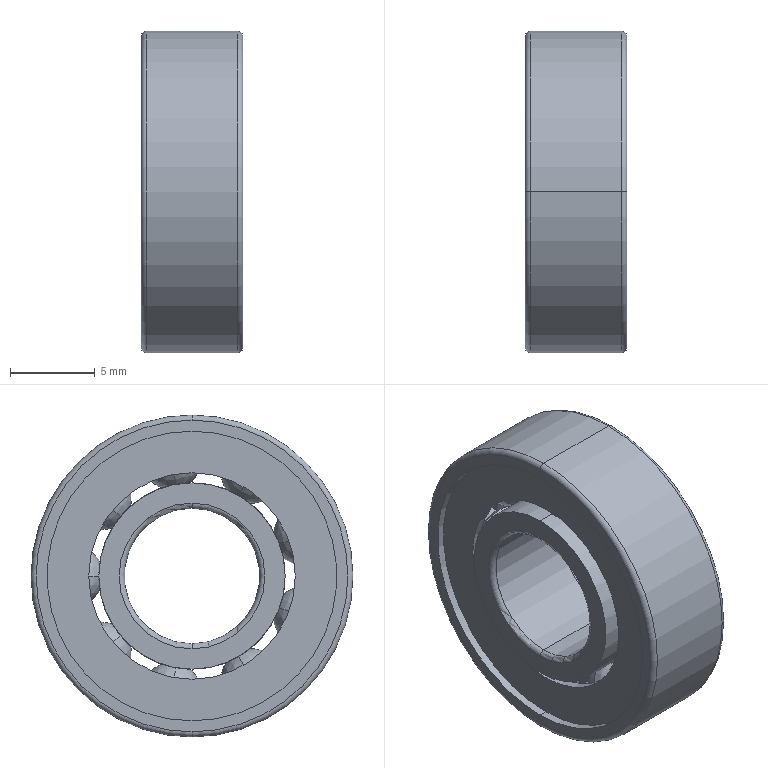Part | STEP file | Deep groove ball bearing 698ZZ | 1 solid | 160 faces | box 6 x 19 x 19 mm | volume 925.778 mm3 | sphere 72 | torus 38 | plane 26 | cylinder 24 | commonest cylinder face diameters 17.1 x8 11 x4 12.188 x4 8 x2 13.06 x2 15.04 x2